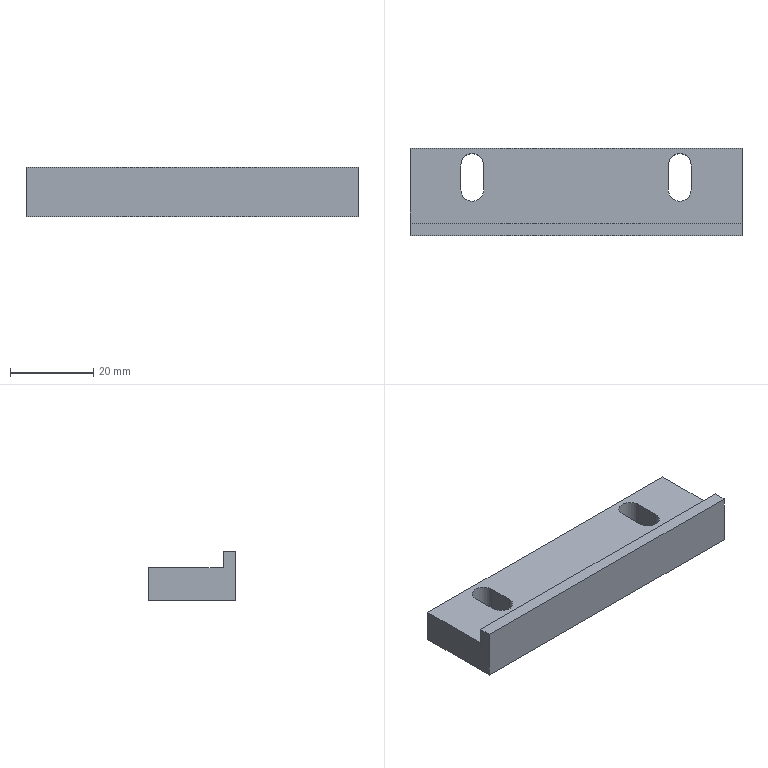Part | SolidWorks | features ICE 2, Extrusion 1, MirrorPattern 1 | 1 solid | 16 faces | box 80 x 21 x 12 mm | volume 13492 mm3 | plane 12 | cylinder 4 | commonest cylinder face diameters 5.5 x4
STEP:
#1=CARTESIAN_POINT('',(40.,3.,8.));
#2=VERTEX_POINT('',#1);
#3=CARTESIAN_POINT('',(-40.,3.,8.));
#4=VERTEX_POINT('',#3);
#5=CARTESIAN_POINT('',(-40.,3.,8.));
#6=DIRECTION('',(-1.,0.,0.));
#7=VECTOR('',#6,1000.);
#8=LINE('',#5,#7);
#9=EDGE_CURVE('',#2,#4,#8,.T.);
#10=ORIENTED_EDGE('',*,*,#9,.F.);
#11=CARTESIAN_POINT('',(40.,21.,8.));
#12=VERTEX_POINT('',#11);
#13=CARTESIAN_POINT('',(40.,21.,8.));
#14=DIRECTION('',(0.,1.,0.));
#15=VECTOR('',#14,1000.);
#16=LINE('',#13,#15);
#17=EDGE_CURVE('',#2,#12,#16,.T.);
#18=ORIENTED_EDGE('',*,*,#17,.T.);
#19=CARTESIAN_POINT('',(-40.,21.,8.));
#20=VERTEX_POINT('',#19);
#21=CARTESIAN_POINT('',(-40.,21.,8.));
#22=DIRECTION('',(-1.,0.,0.));
#23=VECTOR('',#22,1000.);
#24=LINE('',#21,#23);
#25=EDGE_CURVE('',#12,#20,#24,.T.);
#26=ORIENTED_EDGE('',*,*,#25,.T.);
#27=CARTESIAN_POINT('',(-40.,21.,8.));
#28=DIRECTION('',(0.,-1.,0.));
#29=VECTOR('',#28,1000.);
#30=LINE('',#27,#29);
#31=EDGE_CURVE('',#20,#4,#30,.T.);
#32=ORIENTED_EDGE('',*,*,#31,.T.);
#33=EDGE_LOOP('',(#10,#18,#26,#32));
#34=FACE_OUTER_BOUND('',#33,.T.);
#35=CARTESIAN_POINT('',(-22.25,17.,8.));
#36=VERTEX_POINT('',#35);
#37=CARTESIAN_POINT('',(-27.75,17.,8.));
#38=VERTEX_POINT('',#37);
#39=CARTESIAN_POINT('',(-25.,17.,8.));
#40=DIRECTION('',(0.,0.,1.));
#41=DIRECTION('',(1.,0.,0.));
#42=AXIS2_PLACEMENT_3D('',#39,#40,#41);
#43=CIRCLE('',#42,2.75);
#44=EDGE_CURVE('',#36,#38,#43,.T.);
#45=ORIENTED_EDGE('',*,*,#44,.F.);
#46=CARTESIAN_POINT('',(-22.25,11.,8.));
#47=VERTEX_POINT('',#46);
#48=CARTESIAN_POINT('',(-22.25,17.,8.));
#49=DIRECTION('',(0.,1.,0.));
#50=VECTOR('',#49,1000.);
#51=LINE('',#48,#50);
#52=EDGE_CURVE('',#47,#36,#51,.T.);
#53=ORIENTED_EDGE('',*,*,#52,.F.);
#54=CARTESIAN_POINT('',(-27.75,11.,8.));
#55=VERTEX_POINT('',#54);
#56=CARTESIAN_POINT('',(-25.,11.,8.));
#57=DIRECTION('',(0.,0.,1.));
#58=DIRECTION('',(1.,0.,0.));
#59=AXIS2_PLACEMENT_3D('',#56,#57,#58);
#60=CIRCLE('',#59,2.75);
#61=EDGE_CURVE('',#55,#47,#60,.T.);
#62=ORIENTED_EDGE('',*,*,#61,.F.);
#63=CARTESIAN_POINT('',(-27.75,17.,8.));
#64=DIRECTION('',(0.,-1.,0.));
#65=VECTOR('',#64,1000.);
#66=LINE('',#63,#65);
#67=EDGE_CURVE('',#38,#55,#66,.T.);
#68=ORIENTED_EDGE('',*,*,#67,.F.);
#69=EDGE_LOOP('',(#45,#53,#62,#68));
#70=FACE_BOUND('',#69,.T.);
#71=CARTESIAN_POINT('',(22.25,11.,8.));
#72=VERTEX_POINT('',#71);
#73=CARTESIAN_POINT('',(22.25,17.,8.));
#74=VERTEX_POINT('',#73);
#75=CARTESIAN_POINT('',(22.25,17.,8.));
#76=DIRECTION('',(0.,1.,0.));
#77=VECTOR('',#76,1000.);
#78=LINE('',#75,#77);
#79=EDGE_CURVE('',#72,#74,#78,.T.);
#80=ORIENTED_EDGE('',*,*,#79,.T.);
#81=CARTESIAN_POINT('',(27.75,17.,8.));
#82=VERTEX_POINT('',#81);
#83=CARTESIAN_POINT('',(25.,17.,8.));
#84=DIRECTION('',(0.,0.,-1.));
#85=DIRECTION('',(-1.,0.,0.));
#86=AXIS2_PLACEMENT_3D('',#83,#84,#85);
#87=CIRCLE('',#86,2.75);
#88=EDGE_CURVE('',#74,#82,#87,.T.);
#89=ORIENTED_EDGE('',*,*,#88,.T.);
#90=CARTESIAN_POINT('',(27.75,11.,8.));
#91=VERTEX_POINT('',#90);
#92=CARTESIAN_POINT('',(27.75,17.,8.));
#93=DIRECTION('',(0.,-1.,0.));
#94=VECTOR('',#93,1000.);
#95=LINE('',#92,#94);
#96=EDGE_CURVE('',#82,#91,#95,.T.);
#97=ORIENTED_EDGE('',*,*,#96,.T.);
#98=CARTESIAN_POINT('',(25.,11.,8.));
#99=DIRECTION('',(0.,0.,-1.));
#100=DIRECTION('',(-1.,0.,0.));
#101=AXIS2_PLACEMENT_3D('',#98,#99,#100);
#102=CIRCLE('',#101,2.75);
#103=EDGE_CURVE('',#91,#72,#102,.T.);
#104=ORIENTED_EDGE('',*,*,#103,.T.);
#105=EDGE_LOOP('',(#80,#89,#97,#104));
#106=FACE_BOUND('',#105,.T.);
#107=CARTESIAN_POINT('',(0.,0.,8.));
#108=DIRECTION('',(0.,0.,1.));
#109=DIRECTION('',(1.,0.,0.));
#110=AXIS2_PLACEMENT_3D('',#107,#108,#109);
#111=PLANE('',#110);
#112=ADVANCED_FACE('',(#34,#70,#106),#111,.T.);
#113=CARTESIAN_POINT('',(-40.,21.,0.));
#114=VERTEX_POINT('',#113);
#115=CARTESIAN_POINT('',(-40.,0.,0.));
#116=VERTEX_POINT('',#115);
#117=CARTESIAN_POINT('',(-40.,21.,0.));
#118=DIRECTION('',(0.,-1.,0.));
#119=VECTOR('',#118,1000.);
#120=LINE('',#117,#119);
#121=EDGE_CURVE('',#114,#116,#120,.T.);
#122=ORIENTED_EDGE('',*,*,#121,.F.);
#123=CARTESIAN_POINT('',(40.,21.,0.));
#124=VERTEX_POINT('',#123);
#125=CARTESIAN_POINT('',(-40.,21.,0.));
#126=DIRECTION('',(-1.,0.,0.));
#127=VECTOR('',#126,1000.);
#128=LINE('',#125,#127);
#129=EDGE_CURVE('',#124,#114,#128,.T.);
#130=ORIENTED_EDGE('',*,*,#129,.F.);
#131=CARTESIAN_POINT('',(40.,0.,0.));
#132=VERTEX_POINT('',#131);
#133=CARTESIAN_POINT('',(40.,21.,0.));
#134=DIRECTION('',(0.,1.,0.));
#135=VECTOR('',#134,1000.);
#136=LINE('',#133,#135);
#137=EDGE_CURVE('',#132,#124,#136,.T.);
#138=ORIENTED_EDGE('',*,*,#137,.F.);
#139=CARTESIAN_POINT('',(-40.,0.,0.));
#140=DIRECTION('',(1.,0.,0.));
#141=VECTOR('',#140,1000.);
#142=LINE('',#139,#141);
#143=EDGE_CURVE('',#116,#132,#142,.T.);
#144=ORIENTED_EDGE('',*,*,#143,.F.);
#145=EDGE_LOOP('',(#122,#130,#138,#144));
#146=FACE_OUTER_BOUND('',#145,.T.);
#147=CARTESIAN_POINT('',(-22.25,11.,0.));
#148=VERTEX_POINT('',#147);
#149=CARTESIAN_POINT('',(-22.25,17.,0.));
#150=VERTEX_POINT('',#149);
#151=CARTESIAN_POINT('',(-22.25,17.,0.));
#152=DIRECTION('',(0.,1.,0.));
#153=VECTOR('',#152,1000.);
#154=LINE('',#151,#153);
#155=EDGE_CURVE('',#148,#150,#154,.T.);
#156=ORIENTED_EDGE('',*,*,#155,.T.);
#157=CARTESIAN_POINT('',(-27.75,17.,0.));
#158=VERTEX_POINT('',#157);
#159=CARTESIAN_POINT('',(-25.,17.,0.));
#160=DIRECTION('',(0.,0.,1.));
#161=DIRECTION('',(1.,0.,0.));
#162=AXIS2_PLACEMENT_3D('',#159,#160,#161);
#163=CIRCLE('',#162,2.75);
#164=EDGE_CURVE('',#150,#158,#163,.T.);
#165=ORIENTED_EDGE('',*,*,#164,.T.);
#166=CARTESIAN_POINT('',(-27.75,11.,0.));
#167=VERTEX_POINT('',#166);
#168=CARTESIAN_POINT('',(-27.75,17.,0.));
#169=DIRECTION('',(0.,-1.,0.));
#170=VECTOR('',#169,1000.);
#171=LINE('',#168,#170);
#172=EDGE_CURVE('',#158,#167,#171,.T.);
#173=ORIENTED_EDGE('',*,*,#172,.T.);
#174=CARTESIAN_POINT('',(-25.,11.,0.));
#175=DIRECTION('',(0.,0.,1.));
#176=DIRECTION('',(1.,0.,0.));
#177=AXIS2_PLACEMENT_3D('',#174,#175,#176);
#178=CIRCLE('',#177,2.75);
#179=EDGE_CURVE('',#167,#148,#178,.T.);
#180=ORIENTED_EDGE('',*,*,#179,.T.);
#181=EDGE_LOOP('',(#156,#165,#173,#180));
#182=FACE_BOUND('',#181,.T.);
#183=CARTESIAN_POINT('',(22.25,17.,0.));
#184=VERTEX_POINT('',#183);
#185=CARTESIAN_POINT('',(27.75,17.,0.));
#186=VERTEX_POINT('',#185);
#187=CARTESIAN_POINT('',(25.,17.,0.));
#188=DIRECTION('',(0.,0.,-1.));
#189=DIRECTION('',(-1.,0.,0.));
#190=AXIS2_PLACEMENT_3D('',#187,#188,#189);
#191=CIRCLE('',#190,2.75);
#192=EDGE_CURVE('',#184,#186,#191,.T.);
#193=ORIENTED_EDGE('',*,*,#192,.F.);
#194=CARTESIAN_POINT('',(22.25,11.,0.));
#195=VERTEX_POINT('',#194);
#196=CARTESIAN_POINT('',(22.25,17.,0.));
#197=DIRECTION('',(0.,1.,0.));
#198=VECTOR('',#197,1000.);
#199=LINE('',#196,#198);
#200=EDGE_CURVE('',#195,#184,#199,.T.);
#201=ORIENTED_EDGE('',*,*,#200,.F.);
#202=CARTESIAN_POINT('',(27.75,11.,0.));
#203=VERTEX_POINT('',#202);
#204=CARTESIAN_POINT('',(25.,11.,0.));
#205=DIRECTION('',(0.,0.,-1.));
#206=DIRECTION('',(-1.,0.,0.));
#207=AXIS2_PLACEMENT_3D('',#204,#205,#206);
#208=CIRCLE('',#207,2.75);
#209=EDGE_CURVE('',#203,#195,#208,.T.);
#210=ORIENTED_EDGE('',*,*,#209,.F.);
#211=CARTESIAN_POINT('',(27.75,17.,0.));
#212=DIRECTION('',(0.,-1.,0.));
#213=VECTOR('',#212,1000.);
#214=LINE('',#211,#213);
#215=EDGE_CURVE('',#186,#203,#214,.T.);
#216=ORIENTED_EDGE('',*,*,#215,.F.);
#217=EDGE_LOOP('',(#193,#201,#210,#216));
#218=FACE_BOUND('',#217,.T.);
#219=CARTESIAN_POINT('',(0.,0.,0.));
#220=DIRECTION('',(0.,0.,1.));
#221=DIRECTION('',(1.,0.,0.));
#222=AXIS2_PLACEMENT_3D('',#219,#220,#221);
#223=PLANE('',#222);
#224=ADVANCED_FACE('',(#146,#182,#218),#223,.F.);
#225=ORIENTED_EDGE('',*,*,#121,.T.);
#226=CARTESIAN_POINT('',(-40.,0.,12.));
#227=VERTEX_POINT('',#226);
#228=CARTESIAN_POINT('',(-40.,0.,8.));
#229=DIRECTION('',(0.,0.,-1.));
#230=VECTOR('',#229,1000.);
#231=LINE('',#228,#230);
#232=EDGE_CURVE('',#227,#116,#231,.T.);
#233=ORIENTED_EDGE('',*,*,#232,.F.);
#234=CARTESIAN_POINT('',(-40.,3.,12.));
#235=VERTEX_POINT('',#234);
#236=CARTESIAN_POINT('',(-40.,0.,12.));
#237=DIRECTION('',(0.,-1.,0.));
#238=VECTOR('',#237,1000.);
#239=LINE('',#236,#238);
#240=EDGE_CURVE('',#235,#227,#239,.T.);
#241=ORIENTED_EDGE('',*,*,#240,.F.);
#242=CARTESIAN_POINT('',(-40.,3.,12.));
#243=DIRECTION('',(0.,0.,-1.));
#244=VECTOR('',#243,1000.);
#245=LINE('',#242,#244);
#246=EDGE_CURVE('',#235,#4,#245,.T.);
#247=ORIENTED_EDGE('',*,*,#246,.T.);
#248=ORIENTED_EDGE('',*,*,#31,.F.);
#249=CARTESIAN_POINT('',(-40.,21.,8.));
#250=DIRECTION('',(0.,0.,-1.));
#251=VECTOR('',#250,1000.);
#252=LINE('',#249,#251);
#253=EDGE_CURVE('',#20,#114,#252,.T.);
#254=ORIENTED_EDGE('',*,*,#253,.T.);
#255=EDGE_LOOP('',(#225,#233,#241,#247,#248,#254));
#256=FACE_OUTER_BOUND('',#255,.T.);
#257=CARTESIAN_POINT('',(-40.,21.,8.));
#258=DIRECTION('',(1.,0.,0.));
#259=DIRECTION('',(0.,0.,-1.));
#260=AXIS2_PLACEMENT_3D('',#257,#258,#259);
#261=PLANE('',#260);
#262=ADVANCED_FACE('',(#256),#261,.F.);
#263=ORIENTED_EDGE('',*,*,#143,.T.);
#264=CARTESIAN_POINT('',(40.,0.,12.));
#265=VERTEX_POINT('',#264);
#266=CARTESIAN_POINT('',(40.,0.,8.));
#267=DIRECTION('',(0.,0.,-1.));
#268=VECTOR('',#267,1000.);
#269=LINE('',#266,#268);
#270=EDGE_CURVE('',#265,#132,#269,.T.);
#271=ORIENTED_EDGE('',*,*,#270,.F.);
#272=CARTESIAN_POINT('',(-40.,0.,12.));
#273=DIRECTION('',(1.,0.,0.));
#274=VECTOR('',#273,1000.);
#275=LINE('',#272,#274);
#276=EDGE_CURVE('',#227,#265,#275,.T.);
#277=ORIENTED_EDGE('',*,*,#276,.F.);
#278=ORIENTED_EDGE('',*,*,#232,.T.);
#279=EDGE_LOOP('',(#263,#271,#277,#278));
#280=FACE_OUTER_BOUND('',#279,.T.);
#281=CARTESIAN_POINT('',(-40.,0.,8.));
#282=DIRECTION('',(0.,1.,0.));
#283=DIRECTION('',(0.,0.,1.));
#284=AXIS2_PLACEMENT_3D('',#281,#282,#283);
#285=PLANE('',#284);
#286=ADVANCED_FACE('',(#280),#285,.F.);
#287=ORIENTED_EDGE('',*,*,#137,.T.);
#288=CARTESIAN_POINT('',(40.,21.,8.));
#289=DIRECTION('',(0.,0.,-1.));
#290=VECTOR('',#289,1000.);
#291=LINE('',#288,#290);
#292=EDGE_CURVE('',#12,#124,#291,.T.);
#293=ORIENTED_EDGE('',*,*,#292,.F.);
#294=ORIENTED_EDGE('',*,*,#17,.F.);
#295=CARTESIAN_POINT('',(40.,3.,12.));
#296=VERTEX_POINT('',#295);
#297=CARTESIAN_POINT('',(40.,3.,12.));
#298=DIRECTION('',(0.,0.,-1.));
#299=VECTOR('',#298,1000.);
#300=LINE('',#297,#299);
#301=EDGE_CURVE('',#296,#2,#300,.T.);
#302=ORIENTED_EDGE('',*,*,#301,.F.);
#303=CARTESIAN_POINT('',(40.,0.,12.));
#304=DIRECTION('',(0.,1.,0.));
#305=VECTOR('',#304,1000.);
#306=LINE('',#303,#305);
#307=EDGE_CURVE('',#265,#296,#306,.T.);
#308=ORIENTED_EDGE('',*,*,#307,.F.);
#309=ORIENTED_EDGE('',*,*,#270,.T.);
#310=EDGE_LOOP('',(#287,#293,#294,#302,#308,#309));
#311=FACE_OUTER_BOUND('',#310,.T.);
#312=CARTESIAN_POINT('',(40.,21.,8.));
#313=DIRECTION('',(-1.,0.,0.));
#314=DIRECTION('',(0.,0.,1.));
#315=AXIS2_PLACEMENT_3D('',#312,#313,#314);
#316=PLANE('',#315);
#317=ADVANCED_FACE('',(#311),#316,.F.);
#318=ORIENTED_EDGE('',*,*,#129,.T.);
#319=ORIENTED_EDGE('',*,*,#253,.F.);
#320=ORIENTED_EDGE('',*,*,#25,.F.);
#321=ORIENTED_EDGE('',*,*,#292,.T.);
#322=EDGE_LOOP('',(#318,#319,#320,#321));
#323=FACE_OUTER_BOUND('',#322,.T.);
#324=CARTESIAN_POINT('',(-40.,21.,8.));
#325=DIRECTION('',(0.,-1.,0.));
#326=DIRECTION('',(0.,0.,-1.));
#327=AXIS2_PLACEMENT_3D('',#324,#325,#326);
#328=PLANE('',#327);
#329=ADVANCED_FACE('',(#323),#328,.F.);
#330=ORIENTED_EDGE('',*,*,#9,.T.);
#331=ORIENTED_EDGE('',*,*,#246,.F.);
#332=CARTESIAN_POINT('',(-40.,3.,12.));
#333=DIRECTION('',(-1.,0.,0.));
#334=VECTOR('',#333,1000.);
#335=LINE('',#332,#334);
#336=EDGE_CURVE('',#296,#235,#335,.T.);
#337=ORIENTED_EDGE('',*,*,#336,.F.);
#338=ORIENTED_EDGE('',*,*,#301,.T.);
#339=EDGE_LOOP('',(#330,#331,#337,#338));
#340=FACE_OUTER_BOUND('',#339,.T.);
#341=CARTESIAN_POINT('',(-40.,3.,12.));
#342=DIRECTION('',(0.,-1.,0.));
#343=DIRECTION('',(0.,0.,-1.));
#344=AXIS2_PLACEMENT_3D('',#341,#342,#343);
#345=PLANE('',#344);
#346=ADVANCED_FACE('',(#340),#345,.F.);
#347=ORIENTED_EDGE('',*,*,#240,.T.);
#348=ORIENTED_EDGE('',*,*,#276,.T.);
#349=ORIENTED_EDGE('',*,*,#307,.T.);
#350=ORIENTED_EDGE('',*,*,#336,.T.);
#351=EDGE_LOOP('',(#347,#348,#349,#350));
#352=FACE_OUTER_BOUND('',#351,.T.);
#353=CARTESIAN_POINT('',(0.,0.,12.));
#354=DIRECTION('',(0.,0.,-1.));
#355=DIRECTION('',(-1.,0.,0.));
#356=AXIS2_PLACEMENT_3D('',#353,#354,#355);
#357=PLANE('',#356);
#358=ADVANCED_FACE('',(#352),#357,.F.);
#359=ORIENTED_EDGE('',*,*,#44,.T.);
#360=CARTESIAN_POINT('',(-27.75,17.,0.));
#361=DIRECTION('',(0.,0.,1.));
#362=VECTOR('',#361,1000.);
#363=LINE('',#360,#362);
#364=EDGE_CURVE('',#158,#38,#363,.T.);
#365=ORIENTED_EDGE('',*,*,#364,.F.);
#366=ORIENTED_EDGE('',*,*,#164,.F.);
#367=CARTESIAN_POINT('',(-22.25,17.,0.));
#368=DIRECTION('',(0.,0.,1.));
#369=VECTOR('',#368,1000.);
#370=LINE('',#367,#369);
#371=EDGE_CURVE('',#150,#36,#370,.T.);
#372=ORIENTED_EDGE('',*,*,#371,.T.);
#373=EDGE_LOOP('',(#359,#365,#366,#372));
#374=FACE_OUTER_BOUND('',#373,.T.);
#375=CARTESIAN_POINT('',(-25.,17.,0.));
#376=DIRECTION('',(0.,0.,1.));
#377=DIRECTION('',(1.,0.,0.));
#378=AXIS2_PLACEMENT_3D('',#375,#376,#377);
#379=CYLINDRICAL_SURFACE('',#378,2.75);
#380=ADVANCED_FACE('',(#374),#379,.F.);
#381=ORIENTED_EDGE('',*,*,#52,.T.);
#382=ORIENTED_EDGE('',*,*,#371,.F.);
#383=ORIENTED_EDGE('',*,*,#155,.F.);
#384=CARTESIAN_POINT('',(-22.25,11.,0.));
#385=DIRECTION('',(0.,0.,1.));
#386=VECTOR('',#385,1000.);
#387=LINE('',#384,#386);
#388=EDGE_CURVE('',#148,#47,#387,.T.);
#389=ORIENTED_EDGE('',*,*,#388,.T.);
#390=EDGE_LOOP('',(#381,#382,#383,#389));
#391=FACE_OUTER_BOUND('',#390,.T.);
#392=CARTESIAN_POINT('',(-22.25,17.,0.));
#393=DIRECTION('',(1.,0.,0.));
#394=DIRECTION('',(0.,0.,-1.));
#395=AXIS2_PLACEMENT_3D('',#392,#393,#394);
#396=PLANE('',#395);
#397=ADVANCED_FACE('',(#391),#396,.F.);
#398=ORIENTED_EDGE('',*,*,#61,.T.);
#399=ORIENTED_EDGE('',*,*,#388,.F.);
#400=ORIENTED_EDGE('',*,*,#179,.F.);
#401=CARTESIAN_POINT('',(-27.75,11.,0.));
#402=DIRECTION('',(0.,0.,1.));
#403=VECTOR('',#402,1000.);
#404=LINE('',#401,#403);
#405=EDGE_CURVE('',#167,#55,#404,.T.);
#406=ORIENTED_EDGE('',*,*,#405,.T.);
#407=EDGE_LOOP('',(#398,#399,#400,#406));
#408=FACE_OUTER_BOUND('',#407,.T.);
#409=CARTESIAN_POINT('',(-25.,11.,0.));
#410=DIRECTION('',(0.,0.,1.));
#411=DIRECTION('',(1.,0.,0.));
#412=AXIS2_PLACEMENT_3D('',#409,#410,#411);
#413=CYLINDRICAL_SURFACE('',#412,2.75);
#414=ADVANCED_FACE('',(#408),#413,.F.);
#415=ORIENTED_EDGE('',*,*,#67,.T.);
#416=ORIENTED_EDGE('',*,*,#405,.F.);
#417=ORIENTED_EDGE('',*,*,#172,.F.);
#418=ORIENTED_EDGE('',*,*,#364,.T.);
#419=EDGE_LOOP('',(#415,#416,#417,#418));
#420=FACE_OUTER_BOUND('',#419,.T.);
#421=CARTESIAN_POINT('',(-27.75,17.,0.));
#422=DIRECTION('',(-1.,0.,0.));
#423=DIRECTION('',(0.,0.,1.));
#424=AXIS2_PLACEMENT_3D('',#421,#422,#423);
#425=PLANE('',#424);
#426=ADVANCED_FACE('',(#420),#425,.F.);
#427=ORIENTED_EDGE('',*,*,#88,.F.);
#428=CARTESIAN_POINT('',(22.25,17.,0.));
#429=DIRECTION('',(0.,0.,1.));
#430=VECTOR('',#429,1000.);
#431=LINE('',#428,#430);
#432=EDGE_CURVE('',#184,#74,#431,.T.);
#433=ORIENTED_EDGE('',*,*,#432,.F.);
#434=ORIENTED_EDGE('',*,*,#192,.T.);
#435=CARTESIAN_POINT('',(27.75,17.,0.));
#436=DIRECTION('',(0.,0.,1.));
#437=VECTOR('',#436,1000.);
#438=LINE('',#435,#437);
#439=EDGE_CURVE('',#186,#82,#438,.T.);
#440=ORIENTED_EDGE('',*,*,#439,.T.);
#441=EDGE_LOOP('',(#427,#433,#434,#440));
#442=FACE_OUTER_BOUND('',#441,.T.);
#443=CARTESIAN_POINT('',(25.,17.,0.));
#444=DIRECTION('',(0.,0.,1.));
#445=DIRECTION('',(1.,0.,0.));
#446=AXIS2_PLACEMENT_3D('',#443,#444,#445);
#447=CYLINDRICAL_SURFACE('',#446,2.75);
#448=ADVANCED_FACE('',(#442),#447,.F.);
#449=ORIENTED_EDGE('',*,*,#96,.F.);
#450=ORIENTED_EDGE('',*,*,#439,.F.);
#451=ORIENTED_EDGE('',*,*,#215,.T.);
#452=CARTESIAN_POINT('',(27.75,11.,0.));
#453=DIRECTION('',(0.,0.,1.));
#454=VECTOR('',#453,1000.);
#455=LINE('',#452,#454);
#456=EDGE_CURVE('',#203,#91,#455,.T.);
#457=ORIENTED_EDGE('',*,*,#456,.T.);
#458=EDGE_LOOP('',(#449,#450,#451,#457));
#459=FACE_OUTER_BOUND('',#458,.T.);
#460=CARTESIAN_POINT('',(27.75,17.,0.));
#461=DIRECTION('',(-1.,0.,0.));
#462=DIRECTION('',(0.,0.,1.));
#463=AXIS2_PLACEMENT_3D('',#460,#461,#462);
#464=PLANE('',#463);
#465=ADVANCED_FACE('',(#459),#464,.T.);
#466=ORIENTED_EDGE('',*,*,#103,.F.);
#467=ORIENTED_EDGE('',*,*,#456,.F.);
#468=ORIENTED_EDGE('',*,*,#209,.T.);
#469=CARTESIAN_POINT('',(22.25,11.,0.));
#470=DIRECTION('',(0.,0.,1.));
#471=VECTOR('',#470,1000.);
#472=LINE('',#469,#471);
#473=EDGE_CURVE('',#195,#72,#472,.T.);
#474=ORIENTED_EDGE('',*,*,#473,.T.);
#475=EDGE_LOOP('',(#466,#467,#468,#474));
#476=FACE_OUTER_BOUND('',#475,.T.);
#477=CARTESIAN_POINT('',(25.,11.,0.));
#478=DIRECTION('',(0.,0.,1.));
#479=DIRECTION('',(1.,0.,0.));
#480=AXIS2_PLACEMENT_3D('',#477,#478,#479);
#481=CYLINDRICAL_SURFACE('',#480,2.75);
#482=ADVANCED_FACE('',(#476),#481,.F.);
#483=ORIENTED_EDGE('',*,*,#79,.F.);
#484=ORIENTED_EDGE('',*,*,#473,.F.);
#485=ORIENTED_EDGE('',*,*,#200,.T.);
#486=ORIENTED_EDGE('',*,*,#432,.T.);
#487=EDGE_LOOP('',(#483,#484,#485,#486));
#488=FACE_OUTER_BOUND('',#487,.T.);
#489=CARTESIAN_POINT('',(22.25,17.,0.));
#490=DIRECTION('',(1.,0.,0.));
#491=DIRECTION('',(0.,0.,-1.));
#492=AXIS2_PLACEMENT_3D('',#489,#490,#491);
#493=PLANE('',#492);
#494=ADVANCED_FACE('',(#488),#493,.T.);
#495=CLOSED_SHELL('',(#112,#224,#262,#286,#317,#329,#346,#358,#380,#397,#414,#426,#448,#465,#482,#494));
#496=MANIFOLD_SOLID_BREP('',#495);
#497=CARTESIAN_POINT('',(0.,0.,0.));
#498=DIRECTION('',(0.,0.,1.));
#499=DIRECTION('',(1.,0.,0.));
#500=AXIS2_PLACEMENT_3D('',#497,#498,#499);
#501=(LENGTH_UNIT()NAMED_UNIT(*)SI_UNIT(.MILLI.,.METRE.));
#502=UNCERTAINTY_MEASURE_WITH_UNIT(LENGTH_MEASURE(0.00001),#501,'','');
#503=(NAMED_UNIT(*)PLANE_ANGLE_UNIT()SI_UNIT($,.RADIAN.));
#504=(NAMED_UNIT(*)SI_UNIT($,.STERADIAN.)SOLID_ANGLE_UNIT());
#505=(GEOMETRIC_REPRESENTATION_CONTEXT(3)GLOBAL_UNCERTAINTY_ASSIGNED_CONTEXT((#502))GLOBAL_UNIT_ASSIGNED_CONTEXT((#501,#503,#504))REPRESENTATION_CONTEXT('',''));
#506=ADVANCED_BREP_SHAPE_REPRESENTATION('',(#496,#500),#505);